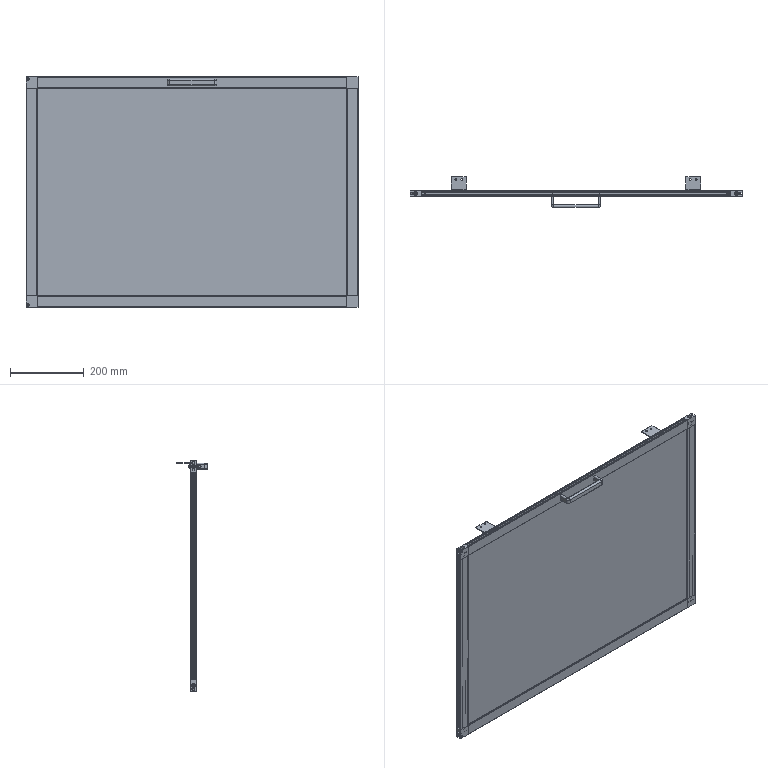Part | SolidWorks | features ReferencePattern 5, LocalLPattern 1 | 30 solids | 1032 faces | box 902 x 84 x 625 mm | volume 3238320 mm3 | plane 610 | cylinder 274 | cone 92 | spline 56 | commonest cylinder face diameters 5 x48 11 x48 4.5 x32 1 x24 3.3 x20 2 x16